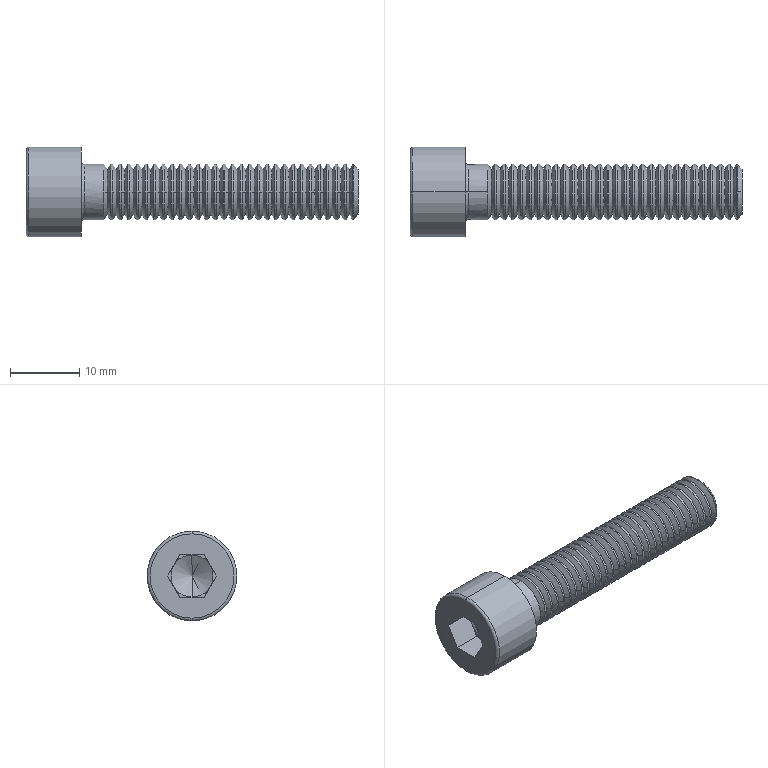Part | STEP file | Socket head screw M8_L16 | 1 solid | 201 faces | box 48 x 13 x 13 mm | volume 2691 mm3 | cone 120 | cylinder 62 | plane 15 | torus 4 | commonest cylinder face diameters 8 x60 13 x2